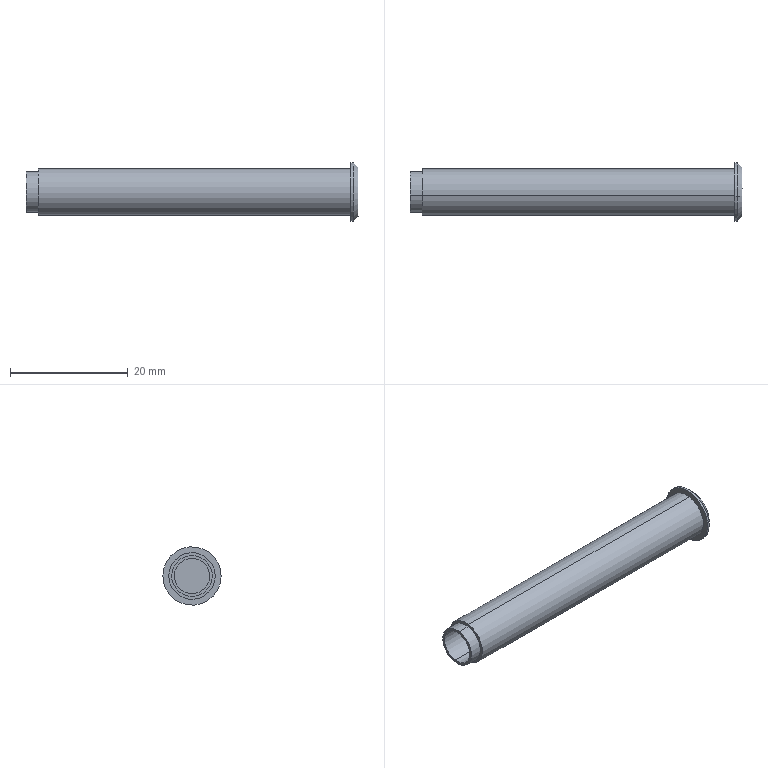Part | SolidWorks | features BaseBody 1 | 1 solid | 15 faces | box 56.3 x 9.9 x 9.9 mm | volume 2448 mm3 | cylinder 8 | plane 5 | cone 2 | commonest cylinder face diameters 6 x2 6.9 x2 7.9 x2 9.9 x2
STEP:
#1=CARTESIAN_POINT('',(-394.545,509.936,-862.063));
#2=VERTEX_POINT('',#1);
#3=CARTESIAN_POINT('',(-394.545,510.851,-867.992));
#4=VERTEX_POINT('',#3);
#5=CARTESIAN_POINT('',(-394.545,510.393,-865.027));
#6=DIRECTION('',(1.,0.,0.));
#7=DIRECTION('',(0.,-0.1525,0.9883));
#8=AXIS2_PLACEMENT_3D('',#5,#6,#7);
#9=CIRCLE('',#8,3.);
#10=EDGE_CURVE('',#2,#4,#9,.T.);
#11=ORIENTED_EDGE('',*,*,#10,.F.);
#12=CARTESIAN_POINT('',(-394.545,510.393,-865.027));
#13=DIRECTION('',(1.,0.,0.));
#14=DIRECTION('',(0.,0.1525,-0.9883));
#15=AXIS2_PLACEMENT_3D('',#12,#13,#14);
#16=CIRCLE('',#15,3.);
#17=EDGE_CURVE('',#4,#2,#16,.T.);
#18=ORIENTED_EDGE('',*,*,#17,.F.);
#19=EDGE_LOOP('',(#11,#18));
#20=FACE_OUTER_BOUND('',#19,.T.);
#21=CARTESIAN_POINT('',(-394.545,510.393,-865.027));
#22=DIRECTION('',(-1.,0.,0.));
#23=DIRECTION('',(0.,0.,1.));
#24=AXIS2_PLACEMENT_3D('',#21,#22,#23);
#25=PLANE('',#24);
#26=ADVANCED_FACE('',(#20),#25,.T.);
#27=ORIENTED_EDGE('',*,*,#17,.T.);
#28=CARTESIAN_POINT('',(-405.545,509.936,-862.063));
#29=VERTEX_POINT('',#28);
#30=CARTESIAN_POINT('',(-405.545,509.936,-862.063));
#31=DIRECTION('',(1.,0.,0.));
#32=VECTOR('',#31,1000.);
#33=LINE('',#30,#32);
#34=EDGE_CURVE('',#29,#2,#33,.T.);
#35=ORIENTED_EDGE('',*,*,#34,.F.);
#36=CARTESIAN_POINT('',(-405.545,510.851,-867.992));
#37=VERTEX_POINT('',#36);
#38=CARTESIAN_POINT('',(-405.545,510.393,-865.027));
#39=DIRECTION('',(-1.,0.,0.));
#40=DIRECTION('',(0.,-0.1525,0.9883));
#41=AXIS2_PLACEMENT_3D('',#38,#39,#40);
#42=CIRCLE('',#41,3.);
#43=EDGE_CURVE('',#29,#37,#42,.T.);
#44=ORIENTED_EDGE('',*,*,#43,.T.);
#45=CARTESIAN_POINT('',(-405.545,510.851,-867.992));
#46=DIRECTION('',(1.,0.,0.));
#47=VECTOR('',#46,1000.);
#48=LINE('',#45,#47);
#49=EDGE_CURVE('',#37,#4,#48,.T.);
#50=ORIENTED_EDGE('',*,*,#49,.T.);
#51=EDGE_LOOP('',(#27,#35,#44,#50));
#52=FACE_OUTER_BOUND('',#51,.T.);
#53=CARTESIAN_POINT('',(-346.43,510.393,-865.027));
#54=DIRECTION('',(-1.,0.,0.));
#55=DIRECTION('',(0.,0.1525,-0.9883));
#56=AXIS2_PLACEMENT_3D('',#53,#54,#55);
#57=CYLINDRICAL_SURFACE('',#56,3.);
#58=ADVANCED_FACE('',(#52),#57,.F.);
#59=CARTESIAN_POINT('',(-405.545,510.393,-865.027));
#60=DIRECTION('',(-1.,0.,0.));
#61=DIRECTION('',(0.,0.1525,-0.9883));
#62=AXIS2_PLACEMENT_3D('',#59,#60,#61);
#63=CIRCLE('',#62,3.);
#64=EDGE_CURVE('',#37,#29,#63,.T.);
#65=ORIENTED_EDGE('',*,*,#64,.T.);
#66=ORIENTED_EDGE('',*,*,#34,.T.);
#67=ORIENTED_EDGE('',*,*,#10,.T.);
#68=ORIENTED_EDGE('',*,*,#49,.F.);
#69=EDGE_LOOP('',(#65,#66,#67,#68));
#70=FACE_OUTER_BOUND('',#69,.T.);
#71=CARTESIAN_POINT('',(-346.43,510.393,-865.027));
#72=DIRECTION('',(-1.,0.,0.));
#73=DIRECTION('',(0.,0.1525,-0.9883));
#74=AXIS2_PLACEMENT_3D('',#71,#72,#73);
#75=CYLINDRICAL_SURFACE('',#74,3.);
#76=ADVANCED_FACE('',(#70),#75,.F.);
#77=ORIENTED_EDGE('',*,*,#43,.F.);
#78=ORIENTED_EDGE('',*,*,#64,.F.);
#79=EDGE_LOOP('',(#77,#78));
#80=FACE_BOUND('',#79,.T.);
#81=CARTESIAN_POINT('',(-405.545,509.867,-861.618));
#82=VERTEX_POINT('',#81);
#83=CARTESIAN_POINT('',(-405.545,510.919,-868.437));
#84=VERTEX_POINT('',#83);
#85=CARTESIAN_POINT('',(-405.545,510.393,-865.027));
#86=DIRECTION('',(1.,0.,0.));
#87=DIRECTION('',(0.,-0.1525,0.9883));
#88=AXIS2_PLACEMENT_3D('',#85,#86,#87);
#89=CIRCLE('',#88,3.45);
#90=EDGE_CURVE('',#82,#84,#89,.T.);
#91=ORIENTED_EDGE('',*,*,#90,.F.);
#92=CARTESIAN_POINT('',(-405.545,510.393,-865.027));
#93=DIRECTION('',(1.,0.,0.));
#94=DIRECTION('',(0.,0.1525,-0.9883));
#95=AXIS2_PLACEMENT_3D('',#92,#93,#94);
#96=CIRCLE('',#95,3.45);
#97=EDGE_CURVE('',#84,#82,#96,.T.);
#98=ORIENTED_EDGE('',*,*,#97,.F.);
#99=EDGE_LOOP('',(#91,#98));
#100=FACE_OUTER_BOUND('',#99,.T.);
#101=CARTESIAN_POINT('',(-405.545,510.393,-865.027));
#102=DIRECTION('',(-1.,0.,0.));
#103=DIRECTION('',(0.,0.,1.));
#104=AXIS2_PLACEMENT_3D('',#101,#102,#103);
#105=PLANE('',#104);
#106=ADVANCED_FACE('',(#80,#100),#105,.T.);
#107=ORIENTED_EDGE('',*,*,#97,.T.);
#108=CARTESIAN_POINT('',(-403.445,509.867,-861.618));
#109=VERTEX_POINT('',#108);
#110=CARTESIAN_POINT('',(-403.445,509.867,-861.618));
#111=DIRECTION('',(-1.,0.,0.));
#112=VECTOR('',#111,1000.);
#113=LINE('',#110,#112);
#114=EDGE_CURVE('',#109,#82,#113,.T.);
#115=ORIENTED_EDGE('',*,*,#114,.F.);
#116=CARTESIAN_POINT('',(-403.445,510.919,-868.437));
#117=VERTEX_POINT('',#116);
#118=CARTESIAN_POINT('',(-403.445,510.393,-865.027));
#119=DIRECTION('',(-1.,0.,0.));
#120=DIRECTION('',(0.,-0.1525,0.9883));
#121=AXIS2_PLACEMENT_3D('',#118,#119,#120);
#122=CIRCLE('',#121,3.45);
#123=EDGE_CURVE('',#109,#117,#122,.T.);
#124=ORIENTED_EDGE('',*,*,#123,.T.);
#125=CARTESIAN_POINT('',(-403.445,510.919,-868.437));
#126=DIRECTION('',(-1.,0.,0.));
#127=VECTOR('',#126,1000.);
#128=LINE('',#125,#127);
#129=EDGE_CURVE('',#117,#84,#128,.T.);
#130=ORIENTED_EDGE('',*,*,#129,.T.);
#131=EDGE_LOOP('',(#107,#115,#124,#130));
#132=FACE_OUTER_BOUND('',#131,.T.);
#133=CARTESIAN_POINT('',(-346.43,510.393,-865.027));
#134=DIRECTION('',(-1.,0.,0.));
#135=DIRECTION('',(0.,0.1525,-0.9883));
#136=AXIS2_PLACEMENT_3D('',#133,#134,#135);
#137=CYLINDRICAL_SURFACE('',#136,3.45);
#138=ADVANCED_FACE('',(#132),#137,.T.);
#139=CARTESIAN_POINT('',(-403.445,510.393,-865.027));
#140=DIRECTION('',(-1.,0.,0.));
#141=DIRECTION('',(0.,0.1525,-0.9883));
#142=AXIS2_PLACEMENT_3D('',#139,#140,#141);
#143=CIRCLE('',#142,3.45);
#144=EDGE_CURVE('',#117,#109,#143,.T.);
#145=ORIENTED_EDGE('',*,*,#144,.T.);
#146=ORIENTED_EDGE('',*,*,#114,.T.);
#147=ORIENTED_EDGE('',*,*,#90,.T.);
#148=ORIENTED_EDGE('',*,*,#129,.F.);
#149=EDGE_LOOP('',(#145,#146,#147,#148));
#150=FACE_OUTER_BOUND('',#149,.T.);
#151=CARTESIAN_POINT('',(-346.43,510.393,-865.027));
#152=DIRECTION('',(-1.,0.,0.));
#153=DIRECTION('',(0.,0.1525,-0.9883));
#154=AXIS2_PLACEMENT_3D('',#151,#152,#153);
#155=CYLINDRICAL_SURFACE('',#154,3.45);
#156=ADVANCED_FACE('',(#150),#155,.T.);
#157=ORIENTED_EDGE('',*,*,#123,.F.);
#158=ORIENTED_EDGE('',*,*,#144,.F.);
#159=EDGE_LOOP('',(#157,#158));
#160=FACE_BOUND('',#159,.T.);
#161=CARTESIAN_POINT('',(-403.445,509.791,-861.124));
#162=VERTEX_POINT('',#161);
#163=CARTESIAN_POINT('',(-403.445,510.995,-868.931));
#164=VERTEX_POINT('',#163);
#165=CARTESIAN_POINT('',(-403.445,510.393,-865.027));
#166=DIRECTION('',(1.,0.,0.));
#167=DIRECTION('',(0.,-0.1525,0.9883));
#168=AXIS2_PLACEMENT_3D('',#165,#166,#167);
#169=CIRCLE('',#168,3.95);
#170=EDGE_CURVE('',#162,#164,#169,.T.);
#171=ORIENTED_EDGE('',*,*,#170,.F.);
#172=CARTESIAN_POINT('',(-403.445,510.393,-865.027));
#173=DIRECTION('',(1.,0.,0.));
#174=DIRECTION('',(0.,0.1525,-0.9883));
#175=AXIS2_PLACEMENT_3D('',#172,#173,#174);
#176=CIRCLE('',#175,3.95);
#177=EDGE_CURVE('',#164,#162,#176,.T.);
#178=ORIENTED_EDGE('',*,*,#177,.F.);
#179=EDGE_LOOP('',(#171,#178));
#180=FACE_OUTER_BOUND('',#179,.T.);
#181=CARTESIAN_POINT('',(-403.445,510.393,-865.027));
#182=DIRECTION('',(-1.,0.,0.));
#183=DIRECTION('',(0.,0.,1.));
#184=AXIS2_PLACEMENT_3D('',#181,#182,#183);
#185=PLANE('',#184);
#186=ADVANCED_FACE('',(#160,#180),#185,.T.);
#187=ORIENTED_EDGE('',*,*,#177,.T.);
#188=CARTESIAN_POINT('',(-350.445,509.791,-861.124));
#189=VERTEX_POINT('',#188);
#190=CARTESIAN_POINT('',(-350.445,509.791,-861.124));
#191=DIRECTION('',(-1.,0.,0.));
#192=VECTOR('',#191,1000.);
#193=LINE('',#190,#192);
#194=EDGE_CURVE('',#189,#162,#193,.T.);
#195=ORIENTED_EDGE('',*,*,#194,.F.);
#196=CARTESIAN_POINT('',(-350.445,510.995,-868.931));
#197=VERTEX_POINT('',#196);
#198=CARTESIAN_POINT('',(-350.445,510.393,-865.027));
#199=DIRECTION('',(-1.,0.,0.));
#200=DIRECTION('',(0.,-0.1525,0.9883));
#201=AXIS2_PLACEMENT_3D('',#198,#199,#200);
#202=CIRCLE('',#201,3.95);
#203=EDGE_CURVE('',#189,#197,#202,.T.);
#204=ORIENTED_EDGE('',*,*,#203,.T.);
#205=CARTESIAN_POINT('',(-350.445,510.995,-868.931));
#206=DIRECTION('',(-1.,0.,0.));
#207=VECTOR('',#206,1000.);
#208=LINE('',#205,#207);
#209=EDGE_CURVE('',#197,#164,#208,.T.);
#210=ORIENTED_EDGE('',*,*,#209,.T.);
#211=EDGE_LOOP('',(#187,#195,#204,#210));
#212=FACE_OUTER_BOUND('',#211,.T.);
#213=CARTESIAN_POINT('',(-346.43,510.393,-865.027));
#214=DIRECTION('',(-1.,0.,0.));
#215=DIRECTION('',(0.,0.1525,-0.9883));
#216=AXIS2_PLACEMENT_3D('',#213,#214,#215);
#217=CYLINDRICAL_SURFACE('',#216,3.95);
#218=ADVANCED_FACE('',(#212),#217,.T.);
#219=CARTESIAN_POINT('',(-350.445,510.393,-865.027));
#220=DIRECTION('',(-1.,0.,0.));
#221=DIRECTION('',(0.,0.1525,-0.9883));
#222=AXIS2_PLACEMENT_3D('',#219,#220,#221);
#223=CIRCLE('',#222,3.95);
#224=EDGE_CURVE('',#197,#189,#223,.T.);
#225=ORIENTED_EDGE('',*,*,#224,.T.);
#226=ORIENTED_EDGE('',*,*,#194,.T.);
#227=ORIENTED_EDGE('',*,*,#170,.T.);
#228=ORIENTED_EDGE('',*,*,#209,.F.);
#229=EDGE_LOOP('',(#225,#226,#227,#228));
#230=FACE_OUTER_BOUND('',#229,.T.);
#231=CARTESIAN_POINT('',(-346.43,510.393,-865.027));
#232=DIRECTION('',(-1.,0.,0.));
#233=DIRECTION('',(0.,0.1525,-0.9883));
#234=AXIS2_PLACEMENT_3D('',#231,#232,#233);
#235=CYLINDRICAL_SURFACE('',#234,3.95);
#236=ADVANCED_FACE('',(#230),#235,.T.);
#237=ORIENTED_EDGE('',*,*,#203,.F.);
#238=ORIENTED_EDGE('',*,*,#224,.F.);
#239=EDGE_LOOP('',(#237,#238));
#240=FACE_BOUND('',#239,.T.);
#241=CARTESIAN_POINT('',(-350.445,509.638,-860.135));
#242=VERTEX_POINT('',#241);
#243=CARTESIAN_POINT('',(-350.445,511.148,-869.92));
#244=VERTEX_POINT('',#243);
#245=CARTESIAN_POINT('',(-350.445,510.393,-865.027));
#246=DIRECTION('',(1.,0.,0.));
#247=DIRECTION('',(0.,-0.1525,0.9883));
#248=AXIS2_PLACEMENT_3D('',#245,#246,#247);
#249=CIRCLE('',#248,4.95);
#250=EDGE_CURVE('',#242,#244,#249,.T.);
#251=ORIENTED_EDGE('',*,*,#250,.F.);
#252=CARTESIAN_POINT('',(-350.445,510.393,-865.027));
#253=DIRECTION('',(1.,0.,0.));
#254=DIRECTION('',(0.,0.1525,-0.9883));
#255=AXIS2_PLACEMENT_3D('',#252,#253,#254);
#256=CIRCLE('',#255,4.95);
#257=EDGE_CURVE('',#244,#242,#256,.T.);
#258=ORIENTED_EDGE('',*,*,#257,.F.);
#259=EDGE_LOOP('',(#251,#258));
#260=FACE_OUTER_BOUND('',#259,.T.);
#261=CARTESIAN_POINT('',(-350.445,510.393,-865.027));
#262=DIRECTION('',(-1.,0.,0.));
#263=DIRECTION('',(0.,0.,1.));
#264=AXIS2_PLACEMENT_3D('',#261,#262,#263);
#265=PLANE('',#264);
#266=ADVANCED_FACE('',(#240,#260),#265,.T.);
#267=ORIENTED_EDGE('',*,*,#257,.T.);
#268=CARTESIAN_POINT('',(-350.045,509.638,-860.135));
#269=VERTEX_POINT('',#268);
#270=CARTESIAN_POINT('',(-350.045,509.638,-860.135));
#271=DIRECTION('',(-1.,0.,0.));
#272=VECTOR('',#271,1000.);
#273=LINE('',#270,#272);
#274=EDGE_CURVE('',#269,#242,#273,.T.);
#275=ORIENTED_EDGE('',*,*,#274,.F.);
#276=CARTESIAN_POINT('',(-350.045,511.148,-869.92));
#277=VERTEX_POINT('',#276);
#278=CARTESIAN_POINT('',(-350.045,510.393,-865.027));
#279=DIRECTION('',(-1.,0.,0.));
#280=DIRECTION('',(0.,-0.1525,0.9883));
#281=AXIS2_PLACEMENT_3D('',#278,#279,#280);
#282=CIRCLE('',#281,4.95);
#283=EDGE_CURVE('',#269,#277,#282,.T.);
#284=ORIENTED_EDGE('',*,*,#283,.T.);
#285=CARTESIAN_POINT('',(-350.045,511.148,-869.92));
#286=DIRECTION('',(-1.,0.,0.));
#287=VECTOR('',#286,1000.);
#288=LINE('',#285,#287);
#289=EDGE_CURVE('',#277,#244,#288,.T.);
#290=ORIENTED_EDGE('',*,*,#289,.T.);
#291=EDGE_LOOP('',(#267,#275,#284,#290));
#292=FACE_OUTER_BOUND('',#291,.T.);
#293=CARTESIAN_POINT('',(-346.43,510.393,-865.027));
#294=DIRECTION('',(-1.,0.,0.));
#295=DIRECTION('',(0.,0.1525,-0.9883));
#296=AXIS2_PLACEMENT_3D('',#293,#294,#295);
#297=CYLINDRICAL_SURFACE('',#296,4.95);
#298=ADVANCED_FACE('',(#292),#297,.T.);
#299=CARTESIAN_POINT('',(-350.045,510.393,-865.027));
#300=DIRECTION('',(-1.,0.,0.));
#301=DIRECTION('',(0.,0.1525,-0.9883));
#302=AXIS2_PLACEMENT_3D('',#299,#300,#301);
#303=CIRCLE('',#302,4.95);
#304=EDGE_CURVE('',#277,#269,#303,.T.);
#305=ORIENTED_EDGE('',*,*,#304,.T.);
#306=ORIENTED_EDGE('',*,*,#274,.T.);
#307=ORIENTED_EDGE('',*,*,#250,.T.);
#308=ORIENTED_EDGE('',*,*,#289,.F.);
#309=EDGE_LOOP('',(#305,#306,#307,#308));
#310=FACE_OUTER_BOUND('',#309,.T.);
#311=CARTESIAN_POINT('',(-346.43,510.393,-865.027));
#312=DIRECTION('',(-1.,0.,0.));
#313=DIRECTION('',(0.,0.1525,-0.9883));
#314=AXIS2_PLACEMENT_3D('',#311,#312,#313);
#315=CYLINDRICAL_SURFACE('',#314,4.95);
#316=ADVANCED_FACE('',(#310),#315,.T.);
#317=CARTESIAN_POINT('',(-349.245,511.026,-869.129));
#318=VERTEX_POINT('',#317);
#319=CARTESIAN_POINT('',(-349.245,509.76,-860.926));
#320=VERTEX_POINT('',#319);
#321=CARTESIAN_POINT('',(-349.245,510.393,-865.027));
#322=DIRECTION('',(-1.,0.,0.));
#323=DIRECTION('',(0.,0.1525,-0.9883));
#324=AXIS2_PLACEMENT_3D('',#321,#322,#323);
#325=CIRCLE('',#324,4.15);
#326=EDGE_CURVE('',#318,#320,#325,.T.);
#327=ORIENTED_EDGE('',*,*,#326,.T.);
#328=CARTESIAN_POINT('',(-349.245,509.76,-860.926));
#329=DIRECTION('',(-0.7071,-0.1078,0.6988));
#330=VECTOR('',#329,1000.);
#331=LINE('',#328,#330);
#332=EDGE_CURVE('',#320,#269,#331,.T.);
#333=ORIENTED_EDGE('',*,*,#332,.T.);
#334=ORIENTED_EDGE('',*,*,#304,.F.);
#335=CARTESIAN_POINT('',(-349.245,511.026,-869.129));
#336=DIRECTION('',(-0.7071,0.1078,-0.6988));
#337=VECTOR('',#336,1000.);
#338=LINE('',#335,#337);
#339=EDGE_CURVE('',#318,#277,#338,.T.);
#340=ORIENTED_EDGE('',*,*,#339,.F.);
#341=EDGE_LOOP('',(#327,#333,#334,#340));
#342=FACE_OUTER_BOUND('',#341,.T.);
#343=CARTESIAN_POINT('',(-349.645,510.393,-865.027));
#344=DIRECTION('',(-1.,0.,0.));
#345=DIRECTION('',(0.,0.1525,-0.9883));
#346=AXIS2_PLACEMENT_3D('',#343,#344,#345);
#347=CONICAL_SURFACE('',#346,4.55,0.7854);
#348=ADVANCED_FACE('',(#342),#347,.T.);
#349=ORIENTED_EDGE('',*,*,#283,.F.);
#350=ORIENTED_EDGE('',*,*,#332,.F.);
#351=CARTESIAN_POINT('',(-349.245,510.393,-865.027));
#352=DIRECTION('',(-1.,0.,0.));
#353=DIRECTION('',(0.,-0.1525,0.9883));
#354=AXIS2_PLACEMENT_3D('',#351,#352,#353);
#355=CIRCLE('',#354,4.15);
#356=EDGE_CURVE('',#320,#318,#355,.T.);
#357=ORIENTED_EDGE('',*,*,#356,.T.);
#358=ORIENTED_EDGE('',*,*,#339,.T.);
#359=EDGE_LOOP('',(#349,#350,#357,#358));
#360=FACE_OUTER_BOUND('',#359,.T.);
#361=CARTESIAN_POINT('',(-349.645,510.393,-865.027));
#362=DIRECTION('',(-1.,0.,0.));
#363=DIRECTION('',(0.,0.1525,-0.9883));
#364=AXIS2_PLACEMENT_3D('',#361,#362,#363);
#365=CONICAL_SURFACE('',#364,4.55,0.7854);
#366=ADVANCED_FACE('',(#360),#365,.T.);
#367=ORIENTED_EDGE('',*,*,#326,.F.);
#368=ORIENTED_EDGE('',*,*,#356,.F.);
#369=EDGE_LOOP('',(#367,#368));
#370=FACE_OUTER_BOUND('',#369,.T.);
#371=CARTESIAN_POINT('',(-349.245,510.393,-865.027));
#372=DIRECTION('',(-1.,0.,0.));
#373=DIRECTION('',(0.,0.,1.));
#374=AXIS2_PLACEMENT_3D('',#371,#372,#373);
#375=PLANE('',#374);
#376=ADVANCED_FACE('',(#370),#375,.F.);
#377=CLOSED_SHELL('',(#26,#58,#76,#106,#138,#156,#186,#218,#236,#266,#298,#316,#348,#366,#376));
#378=MANIFOLD_SOLID_BREP('',#377);
#379=CARTESIAN_POINT('',(0.,0.,0.));
#380=DIRECTION('',(0.,0.,1.));
#381=DIRECTION('',(1.,0.,0.));
#382=AXIS2_PLACEMENT_3D('',#379,#380,#381);
#383=(LENGTH_UNIT()NAMED_UNIT(*)SI_UNIT(.MILLI.,.METRE.));
#384=UNCERTAINTY_MEASURE_WITH_UNIT(LENGTH_MEASURE(0.00001),#383,'','');
#385=(NAMED_UNIT(*)PLANE_ANGLE_UNIT()SI_UNIT($,.RADIAN.));
#386=(NAMED_UNIT(*)SI_UNIT($,.STERADIAN.)SOLID_ANGLE_UNIT());
#387=(GEOMETRIC_REPRESENTATION_CONTEXT(3)GLOBAL_UNCERTAINTY_ASSIGNED_CONTEXT((#384))GLOBAL_UNIT_ASSIGNED_CONTEXT((#383,#385,#386))REPRESENTATION_CONTEXT('',''));
#388=ADVANCED_BREP_SHAPE_REPRESENTATION('',(#378,#382),#387);